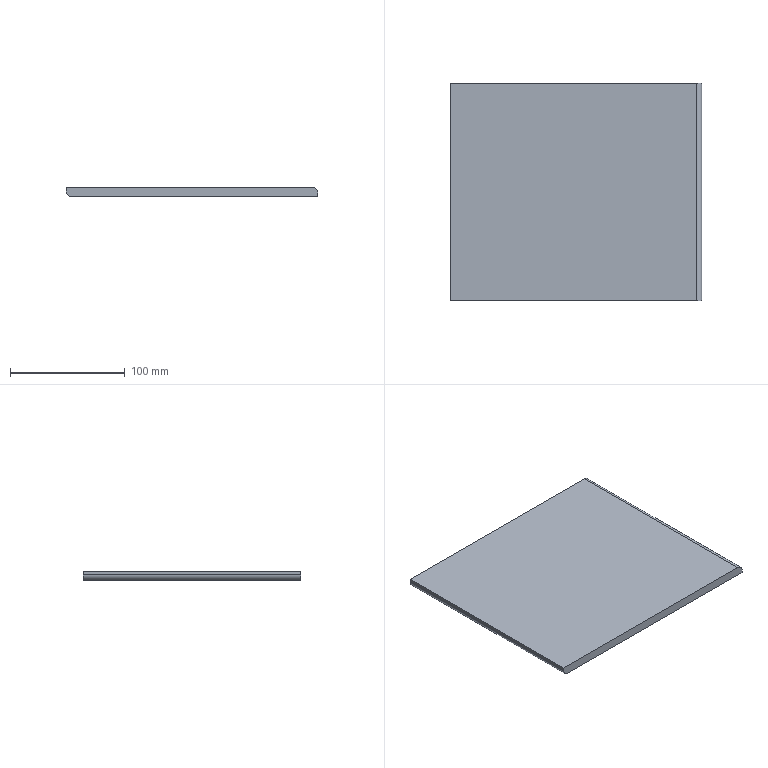Part | SolidWorks | features Extrusion 1, Fillet 1 | 1 solid | 8 faces | box 220 x 190 x 8 mm | volume 332361 mm3 | plane 6 | cylinder 2 | commonest cylinder face diameters 10 x2
STEP:
#1=CARTESIAN_POINT('',(110.,95.,3.));
#2=VERTEX_POINT('',#1);
#3=CARTESIAN_POINT('',(110.,95.,0.));
#4=VERTEX_POINT('',#3);
#5=CARTESIAN_POINT('',(110.,95.,8.));
#6=DIRECTION('',(0.,0.,-1.));
#7=VECTOR('',#6,1000.);
#8=LINE('',#5,#7);
#9=EDGE_CURVE('',#2,#4,#8,.T.);
#10=ORIENTED_EDGE('',*,*,#9,.F.);
#11=CARTESIAN_POINT('',(110.,-95.,3.));
#12=VERTEX_POINT('',#11);
#13=CARTESIAN_POINT('',(110.,-95.,3.));
#14=DIRECTION('',(0.,-1.,0.));
#15=VECTOR('',#14,1000.);
#16=LINE('',#13,#15);
#17=EDGE_CURVE('',#2,#12,#16,.T.);
#18=ORIENTED_EDGE('',*,*,#17,.T.);
#19=CARTESIAN_POINT('',(110.,-95.,0.));
#20=VERTEX_POINT('',#19);
#21=CARTESIAN_POINT('',(110.,-95.,8.));
#22=DIRECTION('',(0.,0.,-1.));
#23=VECTOR('',#22,1000.);
#24=LINE('',#21,#23);
#25=EDGE_CURVE('',#12,#20,#24,.T.);
#26=ORIENTED_EDGE('',*,*,#25,.T.);
#27=CARTESIAN_POINT('',(110.,95.,0.));
#28=DIRECTION('',(0.,1.,0.));
#29=VECTOR('',#28,1000.);
#30=LINE('',#27,#29);
#31=EDGE_CURVE('',#20,#4,#30,.T.);
#32=ORIENTED_EDGE('',*,*,#31,.T.);
#33=EDGE_LOOP('',(#10,#18,#26,#32));
#34=FACE_OUTER_BOUND('',#33,.T.);
#35=CARTESIAN_POINT('',(110.,95.,8.));
#36=DIRECTION('',(-1.,0.,0.));
#37=DIRECTION('',(0.,-1.,0.));
#38=AXIS2_PLACEMENT_3D('',#35,#36,#37);
#39=PLANE('',#38);
#40=ADVANCED_FACE('',(#34),#39,.F.);
#41=CARTESIAN_POINT('',(-105.,95.,0.));
#42=VERTEX_POINT('',#41);
#43=CARTESIAN_POINT('',(-110.,95.,0.));
#44=DIRECTION('',(-1.,0.,0.));
#45=VECTOR('',#44,1000.);
#46=LINE('',#43,#45);
#47=EDGE_CURVE('',#4,#42,#46,.T.);
#48=ORIENTED_EDGE('',*,*,#47,.T.);
#49=CARTESIAN_POINT('',(-110.,95.,5.));
#50=VERTEX_POINT('',#49);
#51=CARTESIAN_POINT('',(-105.,95.,5.));
#52=DIRECTION('',(0.,1.,0.));
#53=DIRECTION('',(0.,0.,-1.));
#54=AXIS2_PLACEMENT_3D('',#51,#52,#53);
#55=CIRCLE('',#54,5.);
#56=EDGE_CURVE('',#42,#50,#55,.T.);
#57=ORIENTED_EDGE('',*,*,#56,.T.);
#58=CARTESIAN_POINT('',(-110.,95.,8.));
#59=VERTEX_POINT('',#58);
#60=CARTESIAN_POINT('',(-110.,95.,8.));
#61=DIRECTION('',(0.,0.,-1.));
#62=VECTOR('',#61,1000.);
#63=LINE('',#60,#62);
#64=EDGE_CURVE('',#59,#50,#63,.T.);
#65=ORIENTED_EDGE('',*,*,#64,.F.);
#66=CARTESIAN_POINT('',(105.,95.,8.));
#67=VERTEX_POINT('',#66);
#68=CARTESIAN_POINT('',(-110.,95.,8.));
#69=DIRECTION('',(-1.,0.,0.));
#70=VECTOR('',#69,1000.);
#71=LINE('',#68,#70);
#72=EDGE_CURVE('',#67,#59,#71,.T.);
#73=ORIENTED_EDGE('',*,*,#72,.F.);
#74=CARTESIAN_POINT('',(105.,95.,3.));
#75=DIRECTION('',(0.,1.,0.));
#76=DIRECTION('',(0.,0.,-1.));
#77=AXIS2_PLACEMENT_3D('',#74,#75,#76);
#78=CIRCLE('',#77,5.);
#79=EDGE_CURVE('',#67,#2,#78,.T.);
#80=ORIENTED_EDGE('',*,*,#79,.T.);
#81=ORIENTED_EDGE('',*,*,#9,.T.);
#82=EDGE_LOOP('',(#48,#57,#65,#73,#80,#81));
#83=FACE_OUTER_BOUND('',#82,.T.);
#84=CARTESIAN_POINT('',(-110.,95.,8.));
#85=DIRECTION('',(0.,-1.,0.));
#86=DIRECTION('',(0.,0.,-1.));
#87=AXIS2_PLACEMENT_3D('',#84,#85,#86);
#88=PLANE('',#87);
#89=ADVANCED_FACE('',(#83),#88,.F.);
#90=ORIENTED_EDGE('',*,*,#64,.T.);
#91=CARTESIAN_POINT('',(-110.,-95.,5.));
#92=VERTEX_POINT('',#91);
#93=CARTESIAN_POINT('',(-110.,95.,5.));
#94=DIRECTION('',(0.,-1.,0.));
#95=VECTOR('',#94,1000.);
#96=LINE('',#93,#95);
#97=EDGE_CURVE('',#50,#92,#96,.T.);
#98=ORIENTED_EDGE('',*,*,#97,.T.);
#99=CARTESIAN_POINT('',(-110.,-95.,8.));
#100=VERTEX_POINT('',#99);
#101=CARTESIAN_POINT('',(-110.,-95.,8.));
#102=DIRECTION('',(0.,0.,-1.));
#103=VECTOR('',#102,1000.);
#104=LINE('',#101,#103);
#105=EDGE_CURVE('',#100,#92,#104,.T.);
#106=ORIENTED_EDGE('',*,*,#105,.F.);
#107=CARTESIAN_POINT('',(-110.,95.,8.));
#108=DIRECTION('',(0.,-1.,0.));
#109=VECTOR('',#108,1000.);
#110=LINE('',#107,#109);
#111=EDGE_CURVE('',#59,#100,#110,.T.);
#112=ORIENTED_EDGE('',*,*,#111,.F.);
#113=EDGE_LOOP('',(#90,#98,#106,#112));
#114=FACE_OUTER_BOUND('',#113,.T.);
#115=CARTESIAN_POINT('',(-110.,95.,8.));
#116=DIRECTION('',(1.,0.,0.));
#117=DIRECTION('',(0.,1.,0.));
#118=AXIS2_PLACEMENT_3D('',#115,#116,#117);
#119=PLANE('',#118);
#120=ADVANCED_FACE('',(#114),#119,.F.);
#121=ORIENTED_EDGE('',*,*,#105,.T.);
#122=CARTESIAN_POINT('',(-105.,-95.,0.));
#123=VERTEX_POINT('',#122);
#124=CARTESIAN_POINT('',(-105.,-95.,5.));
#125=DIRECTION('',(0.,-1.,0.));
#126=DIRECTION('',(0.,0.,1.));
#127=AXIS2_PLACEMENT_3D('',#124,#125,#126);
#128=CIRCLE('',#127,5.);
#129=EDGE_CURVE('',#92,#123,#128,.T.);
#130=ORIENTED_EDGE('',*,*,#129,.T.);
#131=CARTESIAN_POINT('',(-110.,-95.,0.));
#132=DIRECTION('',(1.,0.,0.));
#133=VECTOR('',#132,1000.);
#134=LINE('',#131,#133);
#135=EDGE_CURVE('',#123,#20,#134,.T.);
#136=ORIENTED_EDGE('',*,*,#135,.T.);
#137=ORIENTED_EDGE('',*,*,#25,.F.);
#138=CARTESIAN_POINT('',(105.,-95.,8.));
#139=VERTEX_POINT('',#138);
#140=CARTESIAN_POINT('',(105.,-95.,3.));
#141=DIRECTION('',(0.,-1.,0.));
#142=DIRECTION('',(0.,0.,1.));
#143=AXIS2_PLACEMENT_3D('',#140,#141,#142);
#144=CIRCLE('',#143,5.);
#145=EDGE_CURVE('',#12,#139,#144,.T.);
#146=ORIENTED_EDGE('',*,*,#145,.T.);
#147=CARTESIAN_POINT('',(-110.,-95.,8.));
#148=DIRECTION('',(1.,0.,0.));
#149=VECTOR('',#148,1000.);
#150=LINE('',#147,#149);
#151=EDGE_CURVE('',#100,#139,#150,.T.);
#152=ORIENTED_EDGE('',*,*,#151,.F.);
#153=EDGE_LOOP('',(#121,#130,#136,#137,#146,#152));
#154=FACE_OUTER_BOUND('',#153,.T.);
#155=CARTESIAN_POINT('',(-110.,-95.,8.));
#156=DIRECTION('',(0.,1.,0.));
#157=DIRECTION('',(0.,0.,1.));
#158=AXIS2_PLACEMENT_3D('',#155,#156,#157);
#159=PLANE('',#158);
#160=ADVANCED_FACE('',(#154),#159,.F.);
#161=ORIENTED_EDGE('',*,*,#151,.T.);
#162=CARTESIAN_POINT('',(105.,95.,8.));
#163=DIRECTION('',(0.,1.,0.));
#164=VECTOR('',#163,1000.);
#165=LINE('',#162,#164);
#166=EDGE_CURVE('',#139,#67,#165,.T.);
#167=ORIENTED_EDGE('',*,*,#166,.T.);
#168=ORIENTED_EDGE('',*,*,#72,.T.);
#169=ORIENTED_EDGE('',*,*,#111,.T.);
#170=EDGE_LOOP('',(#161,#167,#168,#169));
#171=FACE_OUTER_BOUND('',#170,.T.);
#172=CARTESIAN_POINT('',(0.,0.,8.));
#173=DIRECTION('',(0.,0.,1.));
#174=DIRECTION('',(1.,0.,0.));
#175=AXIS2_PLACEMENT_3D('',#172,#173,#174);
#176=PLANE('',#175);
#177=ADVANCED_FACE('',(#171),#176,.T.);
#178=ORIENTED_EDGE('',*,*,#135,.F.);
#179=CARTESIAN_POINT('',(-105.,0.,0.));
#180=DIRECTION('',(0.,1.,0.));
#181=VECTOR('',#180,1000.);
#182=LINE('',#179,#181);
#183=EDGE_CURVE('',#123,#42,#182,.T.);
#184=ORIENTED_EDGE('',*,*,#183,.T.);
#185=ORIENTED_EDGE('',*,*,#47,.F.);
#186=ORIENTED_EDGE('',*,*,#31,.F.);
#187=EDGE_LOOP('',(#178,#184,#185,#186));
#188=FACE_OUTER_BOUND('',#187,.T.);
#189=CARTESIAN_POINT('',(0.,0.,0.));
#190=DIRECTION('',(0.,0.,1.));
#191=DIRECTION('',(1.,0.,0.));
#192=AXIS2_PLACEMENT_3D('',#189,#190,#191);
#193=PLANE('',#192);
#194=ADVANCED_FACE('',(#188),#193,.F.);
#195=ORIENTED_EDGE('',*,*,#56,.F.);
#196=ORIENTED_EDGE('',*,*,#183,.F.);
#197=ORIENTED_EDGE('',*,*,#129,.F.);
#198=ORIENTED_EDGE('',*,*,#97,.F.);
#199=EDGE_LOOP('',(#195,#196,#197,#198));
#200=FACE_OUTER_BOUND('',#199,.T.);
#201=CARTESIAN_POINT('',(-105.,95.,5.));
#202=DIRECTION('',(0.,-1.,0.));
#203=DIRECTION('',(1.,0.,0.));
#204=AXIS2_PLACEMENT_3D('',#201,#202,#203);
#205=CYLINDRICAL_SURFACE('',#204,5.);
#206=ADVANCED_FACE('',(#200),#205,.T.);
#207=ORIENTED_EDGE('',*,*,#145,.F.);
#208=ORIENTED_EDGE('',*,*,#17,.F.);
#209=ORIENTED_EDGE('',*,*,#79,.F.);
#210=ORIENTED_EDGE('',*,*,#166,.F.);
#211=EDGE_LOOP('',(#207,#208,#209,#210));
#212=FACE_OUTER_BOUND('',#211,.T.);
#213=CARTESIAN_POINT('',(105.,0.,3.));
#214=DIRECTION('',(0.,-1.,0.));
#215=DIRECTION('',(1.,0.,0.));
#216=AXIS2_PLACEMENT_3D('',#213,#214,#215);
#217=CYLINDRICAL_SURFACE('',#216,5.);
#218=ADVANCED_FACE('',(#212),#217,.T.);
#219=CLOSED_SHELL('',(#40,#89,#120,#160,#177,#194,#206,#218));
#220=MANIFOLD_SOLID_BREP('',#219);
#221=CARTESIAN_POINT('',(0.,0.,0.));
#222=DIRECTION('',(0.,0.,1.));
#223=DIRECTION('',(1.,0.,0.));
#224=AXIS2_PLACEMENT_3D('',#221,#222,#223);
#225=(LENGTH_UNIT()NAMED_UNIT(*)SI_UNIT(.MILLI.,.METRE.));
#226=UNCERTAINTY_MEASURE_WITH_UNIT(LENGTH_MEASURE(0.00001),#225,'','');
#227=(NAMED_UNIT(*)PLANE_ANGLE_UNIT()SI_UNIT($,.RADIAN.));
#228=(NAMED_UNIT(*)SI_UNIT($,.STERADIAN.)SOLID_ANGLE_UNIT());
#229=(GEOMETRIC_REPRESENTATION_CONTEXT(3)GLOBAL_UNCERTAINTY_ASSIGNED_CONTEXT((#226))GLOBAL_UNIT_ASSIGNED_CONTEXT((#225,#227,#228))REPRESENTATION_CONTEXT('',''));
#230=ADVANCED_BREP_SHAPE_REPRESENTATION('',(#220,#224),#229);